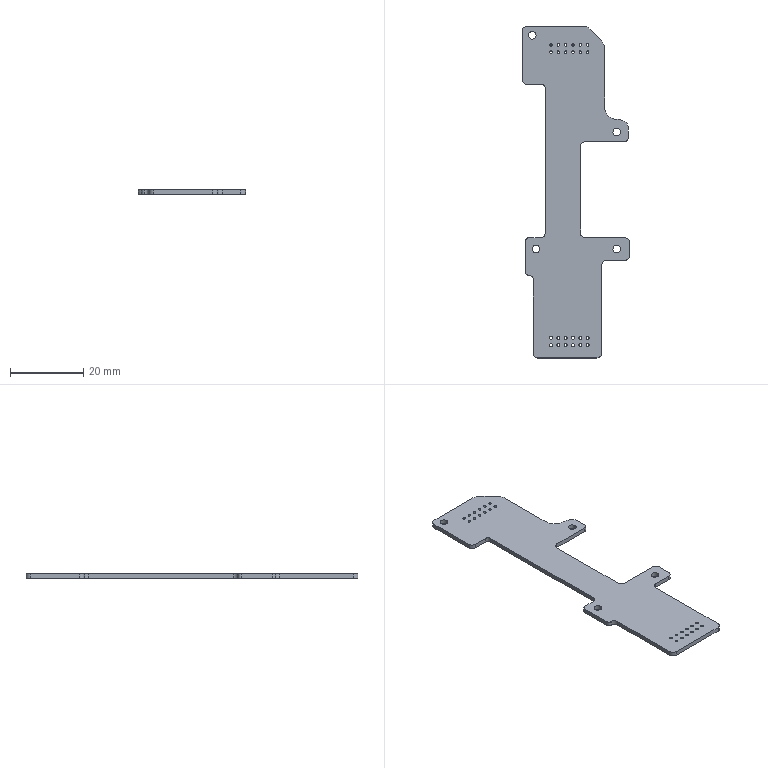Part | STEP file | 推动功放控制2PCB | 1 solid | 70 faces | box 29.18 x 90.51 x 1.2 mm | volume 1855 mm3 | cylinder 49 | plane 21 | commonest cylinder face diameters 0.7 x12 0.8 x12 2.54 x11 6.132 x5 2.1 x4 1.66 x1